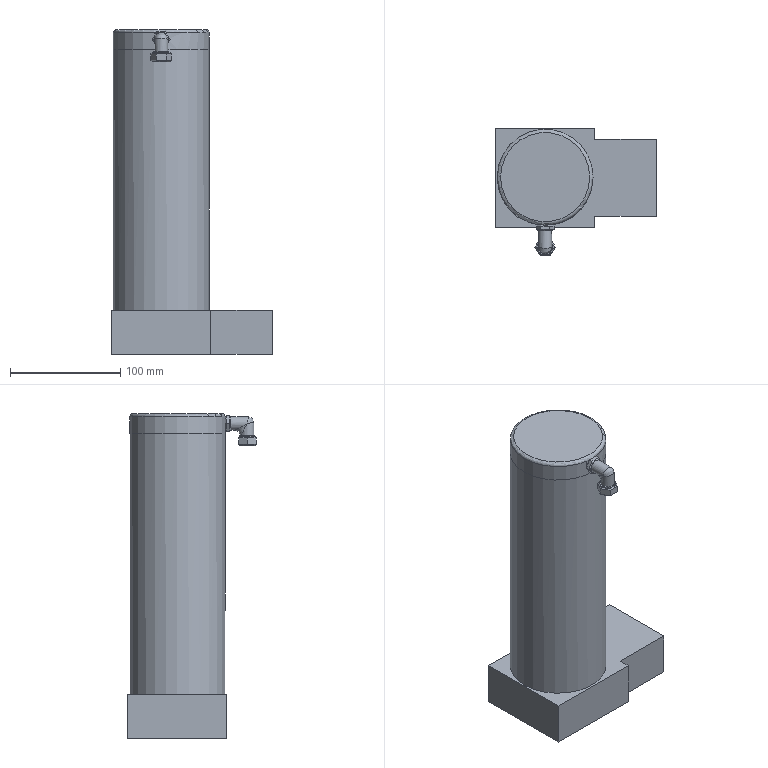Part | STEP file | Tube feed_id750_x_t | 1 solid | 70 faces | box 146 x 116.5 x 295 mm | volume 2001798 mm3 | plane 61 | cylinder 6 | spline 2 | torus 1 | commonest cylinder face diameters 87 x3 12 x2 14 x1